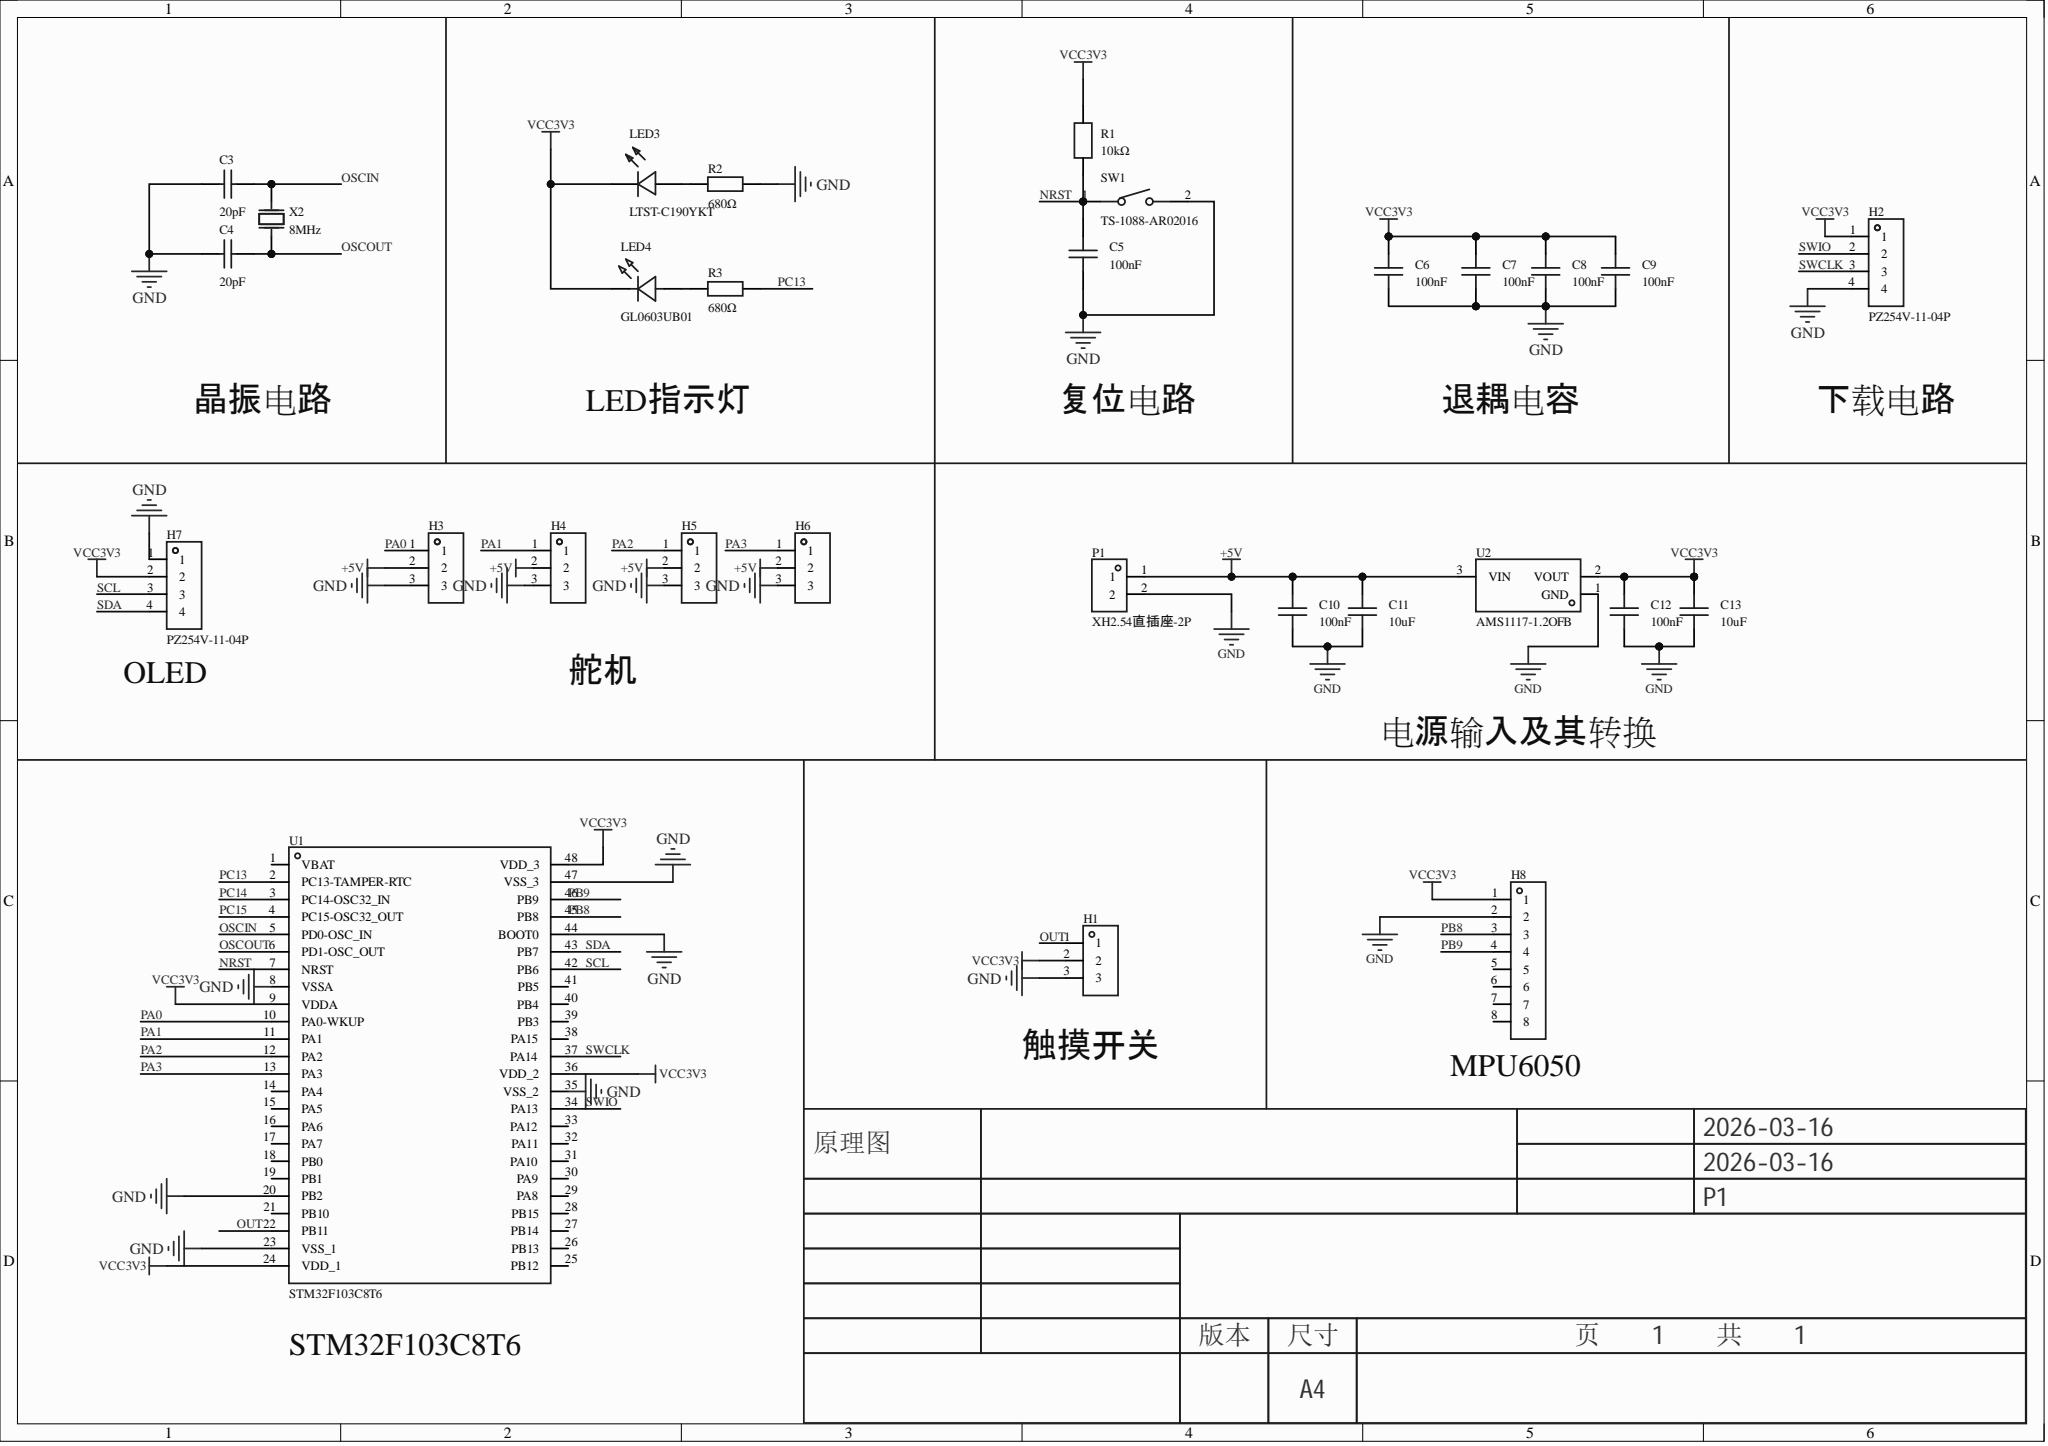Circuit board | Altium Designer | 29 parts | 20 nets
Bill of materials:
Comment,Description,Designator,Footprint,LibRef,Quantity
"20pF","容值:20pF;精度:±5%;额定电压:50V;温度系数:C0G;","C3, C4","C0603","CL10C200JB8NNNC","2"
"100nF","","C5, C6, C7, C8, C9, C10, C12","C0603","CGA0603X7R104K500JT, CAP_0603","7"
"10uF","","C11, C13","C0603","CAP_0603","2"
"","","H1","HDR-TH_3P-P2.54-V-F","HDR-F_2.54_1x3P","1"
"PZ254V-11-04P","插针结构:1x4P;间距:2.54mm;行距:-;圆针/方针:方针;安装方式:直插;排数:单排;总PIN位数:4P;额定电流:3A;额定电压:250V;配合针长度:6mm;塑高:2.5mm;端接针长度:3mm;触头材质:-;工作温度:-40℃~+105℃;颜色:黑色;","H2, H7","HDR-TH_4P-P2.54-V-M","PZ254V-11-04P","2"
"","","H3, H4, H5, H6","HDR-TH_3P-P2.54-V-M","HDR-M_2.54_1x3P","4"
"","","H8","HDR-TH_8P-P2.54-V-F-1","HDR-F_2.54_1x8P","1"
"LTST-C190YKT","发光颜色:黄色;正向压降(Vf):2.1V;功率:60mW;正向电流:20mA;波长:588nm;二极管配置:-;透镜颜色:无色透明透镜;色温:-;发光强度:6mcd;发光角度:130°;载带方式:-;工作温度:-55℃~+85℃;","LED3","LED0603-RD","LTST-C190YKT","1"
"GL0603UB01","发光颜色:蓝色;正向压降(Vf):2.9V;正向电流:20mA;波长:460nm~469nm;二极管配置:独立二极管;透镜颜色:无色透明透镜;发光强度:72mcd;发光角度:120°;载带方式:正贴;工作温度:-40℃~+85℃;","LED4","LED0603-RD_BLUE","GL0603UB01","1"
"XH2.54直插座-2P","","P1","CONN-TH_XH2.54-2P","XH2.54直插座-2P","1"
"10kΩ","","R1","R0603","AST0310KF","1"
"680Ω","","R2, R3","R0603","0603WAF6800T5E","2"
"TS-1088-AR02016","电路结构:单刀单掷;按钮形状:圆形按钮;作用力:1.6N;安装方式:立贴;开关长度:4mm;开关宽度:3mm;开关高度:2mm;带支架:不带支架;触点电流:50mA;额定电压:12V;工作寿命:10万次;","SW1","SW-SMD_L3.9-W3.0-P4.45","TS-1088-AR02016","1"
"STM32F103C8T6","CPU内核:ARM-M3;CPU最大主频:72MHz;应用领域:-;","U1","LQFP-48_L7.0-W7.0-P0.50-LS9.0-BL","STM32F103C8T6","1"
"AMS1117-1.2OFB","输出类型:固定;工作电压:15V;输出电压:1.2V;输出电流:1A;电源纹波抑制比(PSRR):-;输出极性:正极;","U2","SOT-89-3_L4.5-W2.4-P1.50-LS4.0-BR","AMS1117-1.2OFB","1"
"8MHz","晶振类型:贴片晶振;频率:8MHz;常温频差:±10ppm;负载电容:20pF;频率稳定度:±20ppm;","X2","CRYSTAL-SMD_L5.0-W3.2","X50328MSB2GI","1"
Netlist (Protel format):
[
C3
C0603
20pF



]
[
C4
C0603
20pF



]
[
C5
C0603
100nF



]
[
C6
C0603
100nF



]
[
C7
C0603
100nF



]
[
C8
C0603
100nF



]
[
C9
C0603
100nF



]
[
C10
C0603
100nF



]
[
C11
C0603
10uF



]
[
C12
C0603
100nF



]
[
C13
C0603
10uF



]
[
H1
HDR-TH_3P-P2.54-V-F




]
[
H2
HDR-TH_4P-P2.54-V-M
PZ254V-11-04P



]
[
H3
HDR-TH_3P-P2.54-V-M




]
[
H4
HDR-TH_3P-P2.54-V-M




]
[
H5
HDR-TH_3P-P2.54-V-M




]
[
H6
HDR-TH_3P-P2.54-V-M




]
[
H7
HDR-TH_4P-P2.54-V-M
PZ254V-11-04P



]
[
H8
HDR-TH_8P-P2.54-V-F-1




]
[
LED3
LED0603-RD
LTST-C190YKT



]
[
LED4
LED0603-RD_BLUE
GL0603UB01



]
[
P1
CONN-TH_XH2.54-2P
XH2.54直插座-2P



]
[
R1
R0603
10kΩ



]
[
R2
R0603
680Ω



]
[
R3
R0603
680Ω



]
[
SW1
SW-SMD_L3.9-W3.0-P4.45
TS-1088-AR02016



]
[
U1
LQFP-48_L7.0-W7.0-P0.50-LS9.0-BL
STM32F103C8T6



]
[
U2
SOT-89-3_L4.5-W2.4-P1.50-LS4.0-BR
AMS1117-1.2OFB



]
[
X2
CRYSTAL-SMD_L5.0-W3.2
8MHz



]
(
VCC3V3
C6-2
C7-2
C8-2
C9-2
C12-2
C13-2
H1-2
H2-1
H7-2
H8-1
LED3-1
LED4-1
R1-2
U1-9
U1-24
U1-36
U1-48
U2-2
)
(
SWIO
H2-2
U1-34
)
(
SWCLK
H2-3
U1-37
)
(
SDA
H7-4
U1-43
)
(
SCL
H7-3
U1-42
)
(
PC13
R3-2
U1-2
)
(
PB9
H8-4
U1-46
)
(
PB8
H8-3
U1-45
)
(
PA3
H6-1
U1-13
)
(
PA2
H5-1
U1-12
)
(
PA1
H4-1
U1-11
)
(
PA0
H3-1
U1-10
)
(
OUT
H1-1
U1-22
)
(
OSCOUT
C4-2
U1-6
X2-1
)
(
OSCIN
C3-2
U1-5
X2-2
)
(
NRST
C5-2
R1-1
SW1-1
U1-7
)
(
NetLED4_2
LED4-2
R3-1
)
(
NetLED3_2
LED3-2
R2-1
)
(
GND
C3-1
C4-1
C5-1
C6-1
C7-1
C8-1
C9-1
C10-1
C11-1
C12-1
C13-1
H1-3
H2-4
H3-3
H4-3
H5-3
H6-3
H7-1
H8-2
P1-2
R2-2
SW1-2
U1-8
U1-20
U1-23
U1-35
U1-44
U1-47
U2-1
)
(
+5V
C10-2
C11-2
H3-2
H4-2
H5-2
H6-2
P1-1
U2-3
)